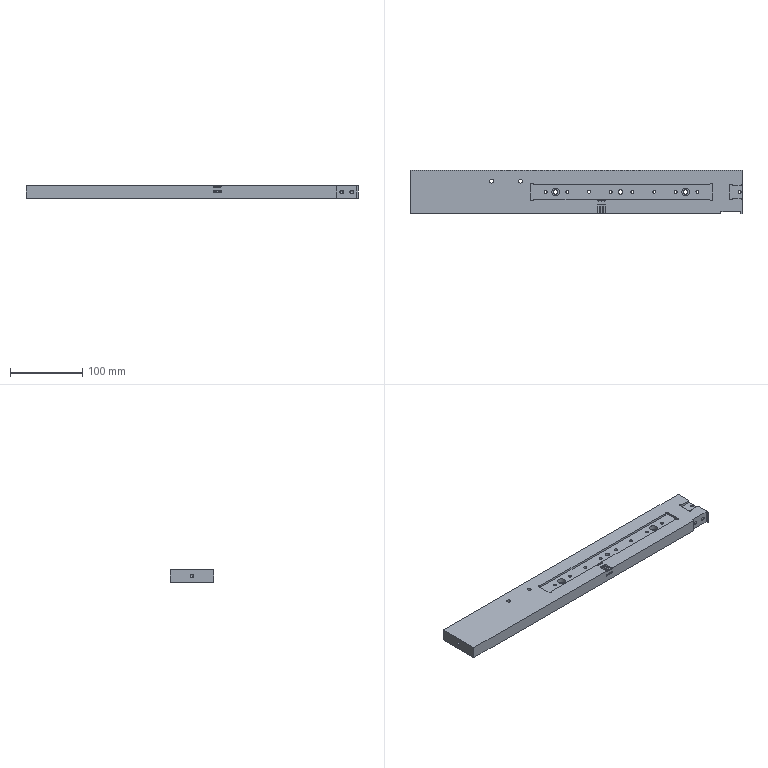Part | NX | 1 solid | 84 faces | box 459.645 x 60 x 17 mm | volume 444065 mm3 | cylinder 38 | plane 23 | cone 23 | commonest cylinder face diameters 4.2 x12 2.5 x9 4 x8 6.4 x3 5.3 x2 9.5 x2